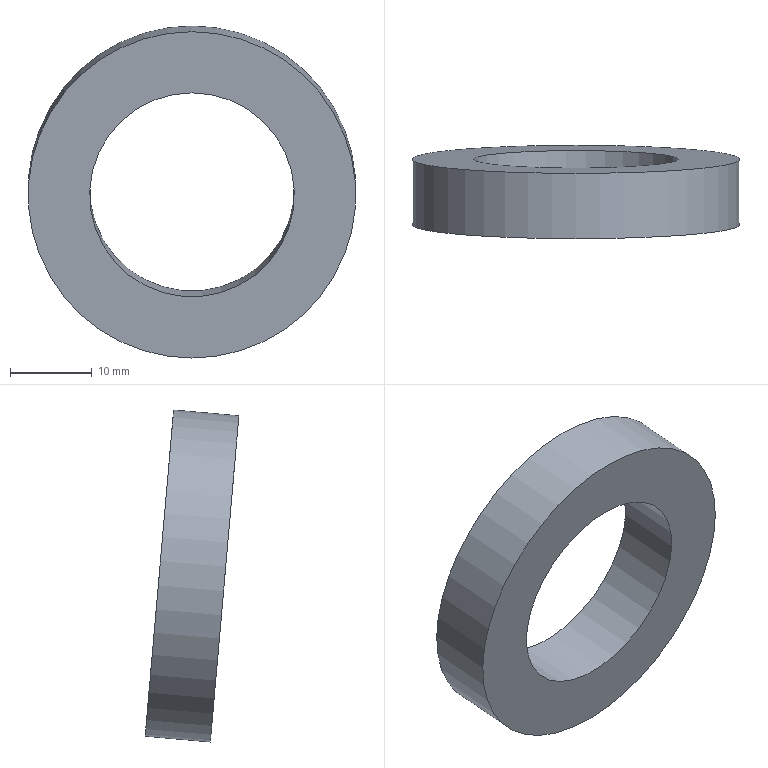Part | NX | features solid 2 | 1 solid | 4 faces | box 40 x 11.456 x 40.545 mm | volume 6126 mm3 | cylinder 2 | plane 2 | commonest cylinder face diameters 25 x1 40 x1
STEP:
#1=CARTESIAN_POINT('',(-150.187,67.538,-16.908));
#2=VERTEX_POINT('',#1);
#3=CARTESIAN_POINT('',(-150.187,69.282,-36.832));
#4=DIRECTION('',(0.,0.9962,0.08716));
#5=DIRECTION('',(0.,-0.08716,0.9962));
#6=AXIS2_PLACEMENT_3D('',#3,#4,#5);
#7=CIRCLE('',#6,20.);
#8=EDGE_CURVE('',#2,#2,#7,.T.);
#9=ORIENTED_EDGE('',*,*,#8,.T.);
#10=EDGE_LOOP('',(#9));
#11=FACE_BOUND('',#10,.T.);
#12=CARTESIAN_POINT('',(-150.187,75.508,-16.211));
#13=VERTEX_POINT('',#12);
#14=CARTESIAN_POINT('',(-150.187,77.251,-36.135));
#15=DIRECTION('',(0.,0.9962,0.08716));
#16=DIRECTION('',(0.,-0.08716,0.9962));
#17=AXIS2_PLACEMENT_3D('',#14,#15,#16);
#18=CIRCLE('',#17,20.);
#19=EDGE_CURVE('',#13,#13,#18,.T.);
#20=ORIENTED_EDGE('',*,*,#19,.F.);
#21=EDGE_LOOP('',(#20));
#22=FACE_BOUND('',#21,.T.);
#23=CARTESIAN_POINT('',(-150.187,69.282,-36.832));
#24=DIRECTION('',(0.,0.9962,0.08716));
#25=DIRECTION('',(0.,-0.08716,0.9962));
#26=AXIS2_PLACEMENT_3D('',#23,#24,#25);
#27=CYLINDRICAL_SURFACE('',#26,20.);
#28=ADVANCED_FACE('',(#11,#22),#27,.T.);
#29=CARTESIAN_POINT('',(-150.187,68.192,-24.379));
#30=VERTEX_POINT('',#29);
#31=CARTESIAN_POINT('',(-150.187,69.282,-36.832));
#32=DIRECTION('',(0.,0.9962,0.08716));
#33=DIRECTION('',(0.,-0.08716,0.9962));
#34=AXIS2_PLACEMENT_3D('',#31,#32,#33);
#35=CIRCLE('',#34,12.5);
#36=EDGE_CURVE('',#30,#30,#35,.T.);
#37=ORIENTED_EDGE('',*,*,#36,.T.);
#38=EDGE_LOOP('',(#37));
#39=FACE_BOUND('',#38,.T.);
#40=ORIENTED_EDGE('',*,*,#8,.F.);
#41=EDGE_LOOP('',(#40));
#42=FACE_BOUND('',#41,.T.);
#43=CARTESIAN_POINT('',(-150.187,69.282,-36.832));
#44=DIRECTION('',(0.,0.9962,0.08716));
#45=DIRECTION('',(0.,-0.08716,0.9962));
#46=AXIS2_PLACEMENT_3D('',#43,#44,#45);
#47=PLANE('',#46);
#48=ADVANCED_FACE('',(#39,#42),#47,.F.);
#49=CARTESIAN_POINT('',(-150.187,76.162,-23.682));
#50=VERTEX_POINT('',#49);
#51=CARTESIAN_POINT('',(-150.187,77.251,-36.135));
#52=DIRECTION('',(0.,0.9962,0.08716));
#53=DIRECTION('',(0.,-0.08716,0.9962));
#54=AXIS2_PLACEMENT_3D('',#51,#52,#53);
#55=CIRCLE('',#54,12.5);
#56=EDGE_CURVE('',#50,#50,#55,.T.);
#57=ORIENTED_EDGE('',*,*,#56,.F.);
#58=EDGE_LOOP('',(#57));
#59=FACE_BOUND('',#58,.T.);
#60=ORIENTED_EDGE('',*,*,#19,.T.);
#61=EDGE_LOOP('',(#60));
#62=FACE_BOUND('',#61,.T.);
#63=CARTESIAN_POINT('',(-150.187,77.251,-36.135));
#64=DIRECTION('',(0.,0.9962,0.08716));
#65=DIRECTION('',(0.,-0.08716,0.9962));
#66=AXIS2_PLACEMENT_3D('',#63,#64,#65);
#67=PLANE('',#66);
#68=ADVANCED_FACE('',(#59,#62),#67,.T.);
#69=ORIENTED_EDGE('',*,*,#56,.T.);
#70=EDGE_LOOP('',(#69));
#71=FACE_BOUND('',#70,.T.);
#72=ORIENTED_EDGE('',*,*,#36,.F.);
#73=EDGE_LOOP('',(#72));
#74=FACE_BOUND('',#73,.T.);
#75=CARTESIAN_POINT('',(-150.187,69.282,-36.832));
#76=DIRECTION('',(0.,0.9962,0.08716));
#77=DIRECTION('',(0.,-0.08716,0.9962));
#78=AXIS2_PLACEMENT_3D('',#75,#76,#77);
#79=CYLINDRICAL_SURFACE('',#78,12.5);
#80=ADVANCED_FACE('',(#71,#74),#79,.F.);
#81=CLOSED_SHELL('',(#28,#48,#68,#80));
#82=MANIFOLD_SOLID_BREP('',#81);
#83=(LENGTH_UNIT()NAMED_UNIT(*)SI_UNIT(.MILLI.,.METRE.));
#84=UNCERTAINTY_MEASURE_WITH_UNIT(LENGTH_MEASURE(0.00001),#83,'','');
#85=(NAMED_UNIT(*)PLANE_ANGLE_UNIT()SI_UNIT($,.RADIAN.));
#86=(NAMED_UNIT(*)SI_UNIT($,.STERADIAN.)SOLID_ANGLE_UNIT());
#87=(GEOMETRIC_REPRESENTATION_CONTEXT(3)GLOBAL_UNCERTAINTY_ASSIGNED_CONTEXT((#84))GLOBAL_UNIT_ASSIGNED_CONTEXT((#83,#85,#86))REPRESENTATION_CONTEXT('',''));
#88=ADVANCED_BREP_SHAPE_REPRESENTATION('',(#82),#87);